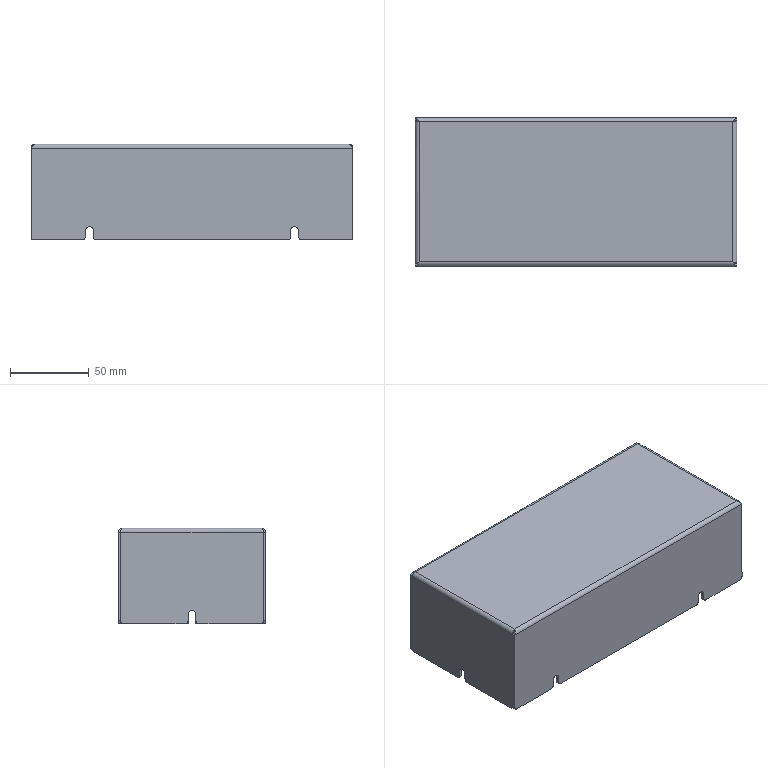Part | SolidWorks | features BaseBody 1 | 1 solid | 82 faces | box 203.7 x 93.7 x 60.5 mm | volume 79662 mm3 | plane 40 | cylinder 34 | spline 8 | commonest cylinder face diameters 4 x18 4.8 x8 2 x4 5 x4